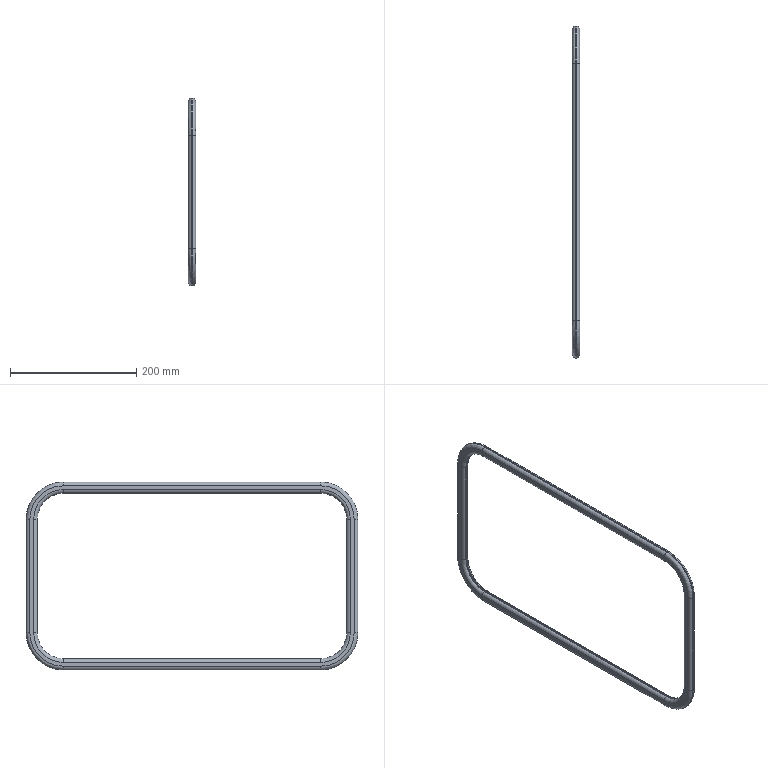Part | STEP file | Part 8^Sheet metal guard | 1 solid | 54 faces | box 12 x 525.906 x 297.906 mm | volume 225066 mm3 | cylinder 24 | torus 16 | plane 14 | commonest cylinder face diameters 12 x16 96 x4 100 x4